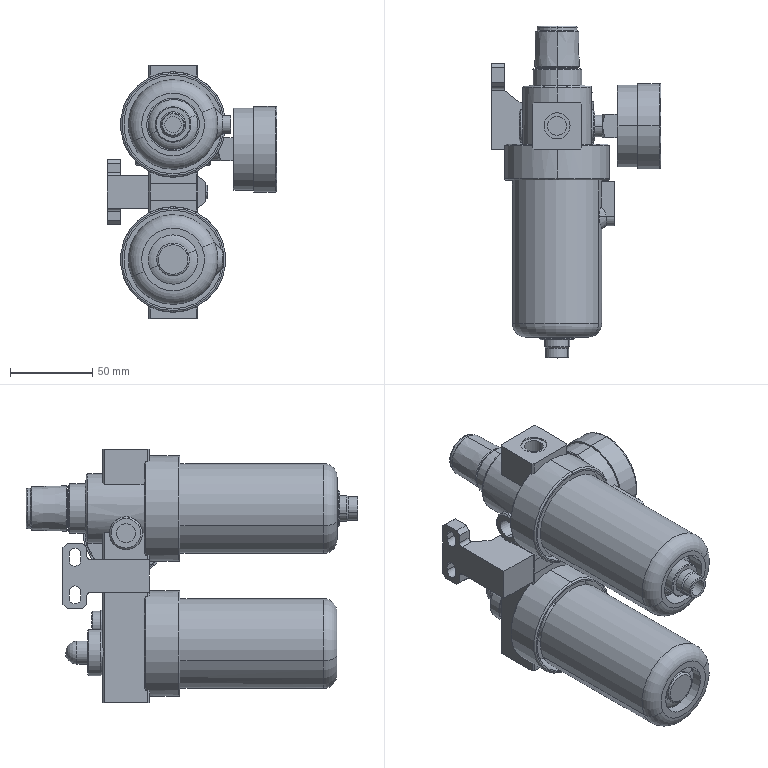Part | SolidWorks | 7 solids | 329 faces | box 103 x 201.6 x 154 mm | volume 430309 mm3 | plane 141 | cylinder 113 | cone 44 | torus 30 | sphere 1 | commonest cylinder face diameters 11.445 x12 20 x10 15.788 x8 7 x6 6 x4 8 x4